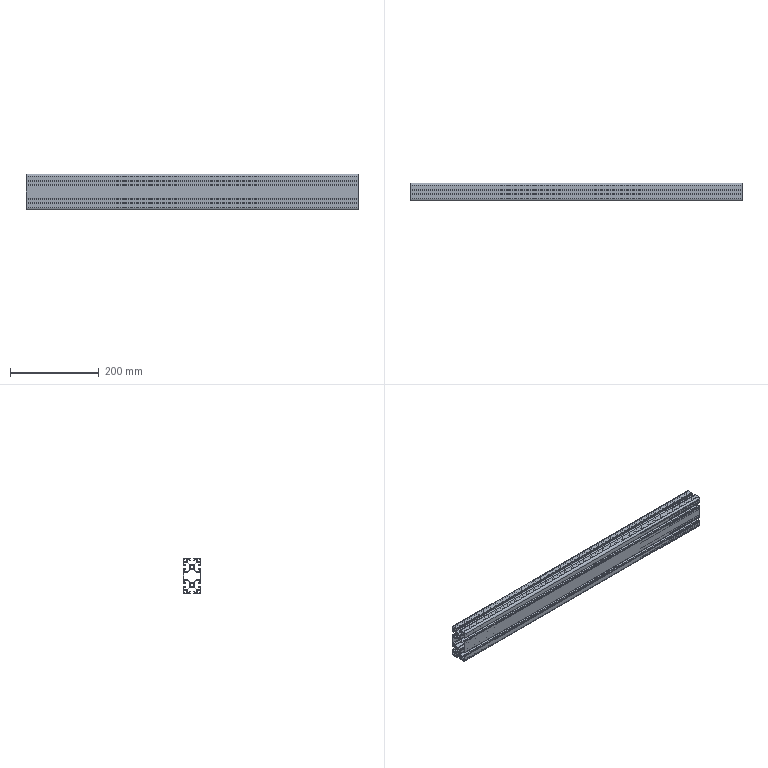Part | STEP file | MK-8-4080H-L-02 Profile 4080H Standard 747mm | 1 solid | 294 faces | box 747 x 40 x 80 mm | volume 606353 mm3 | cylinder 148 | plane 142 | cone 4 | commonest cylinder face diameters 0.6 x44 2 x44 4 x28 0.4 x14 6 x4 6.8 x4